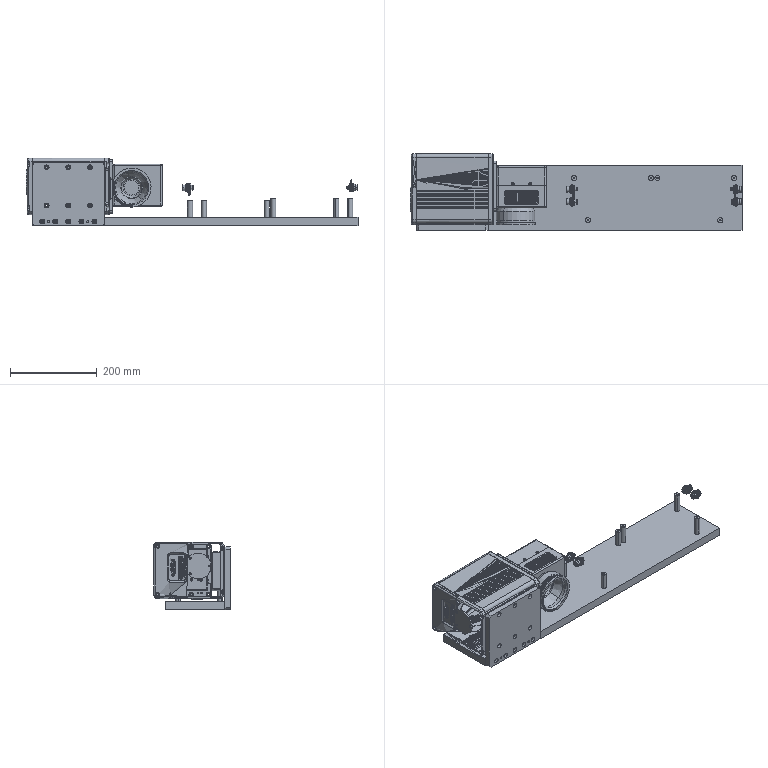Part | NX | features BREP 25 | 26 solids | 2209 faces | box 765 x 176 x 156 mm | volume 741970 mm3 | plane 971 | cylinder 911 | cone 147 | spline 119 | torus 37 | sphere 24 | commonest cylinder face diameters 6 x186 0.7 x96 5 x46 1.1 x44 0.8 x32 1.6 x32